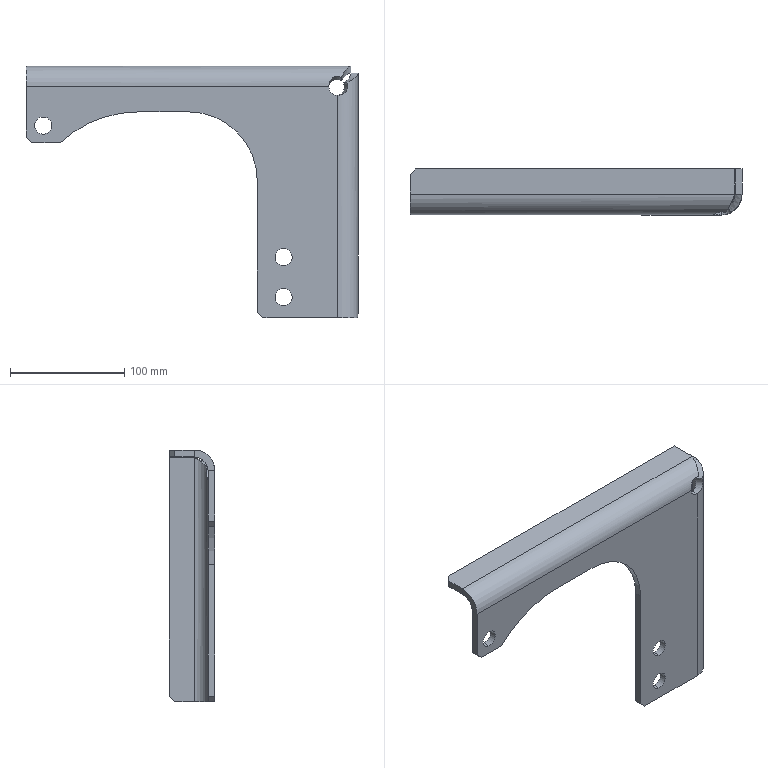Part | SolidWorks | features Chamfer 1, EdgeFlange 1, FlatPattern 1, Fold 1, ICE 1, SMBaseFlange 1, SheetMetal 1, UnFold 1 | 1 solid | 40 faces | box 290 x 40 x 220 mm | volume 254298 mm3 | plane 23 | cylinder 13 | spline 4 | commonest cylinder face diameters 15 x7 24 x2 36 x2 120 x1 200 x1